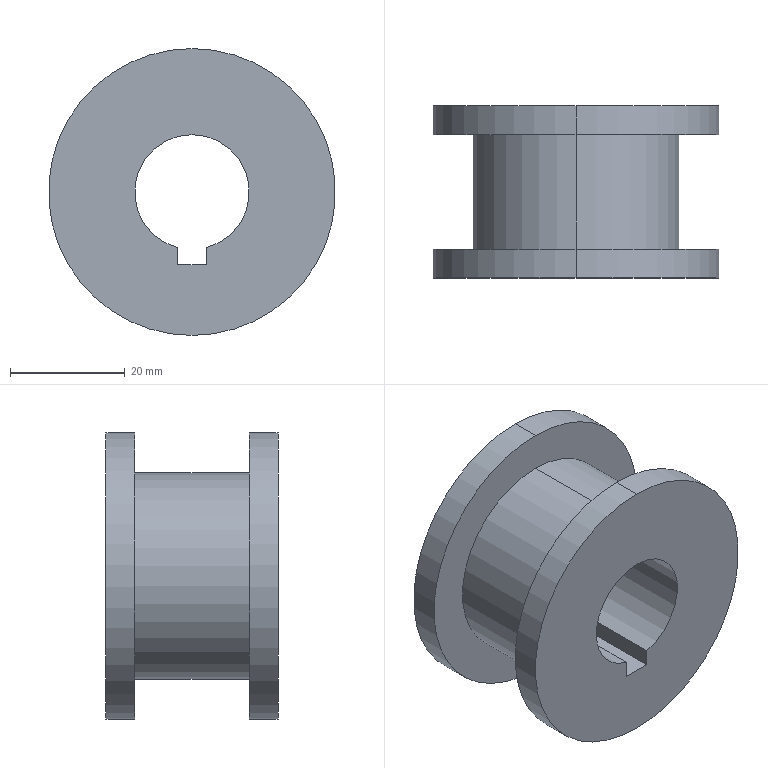Part | SolidWorks | features ICE 1, Revolution 1 | 1 solid | 15 faces | box 50 x 30 x 50 mm | volume 30150 mm3 | cylinder 8 | plane 7 | commonest cylinder face diameters 50 x4 20 x2 36 x2
STEP:
#1=CARTESIAN_POINT('',(0.,-5.,25.));
#2=VERTEX_POINT('',#1);
#3=CARTESIAN_POINT('',(0.,-5.,-25.));
#4=VERTEX_POINT('',#3);
#5=CARTESIAN_POINT('',(0.,-5.,0.));
#6=DIRECTION('',(0.,1.,0.));
#7=DIRECTION('',(0.,0.,1.));
#8=AXIS2_PLACEMENT_3D('',#5,#6,#7);
#9=CIRCLE('',#8,25.);
#10=EDGE_CURVE('',#2,#4,#9,.T.);
#11=ORIENTED_EDGE('',*,*,#10,.T.);
#12=CARTESIAN_POINT('',(0.,0.,-25.));
#13=VERTEX_POINT('',#12);
#14=CARTESIAN_POINT('',(0.,76.759,-25.));
#15=DIRECTION('',(0.,1.,0.));
#16=VECTOR('',#15,1000.);
#17=LINE('',#14,#16);
#18=EDGE_CURVE('',#4,#13,#17,.T.);
#19=ORIENTED_EDGE('',*,*,#18,.T.);
#20=CARTESIAN_POINT('',(0.,0.,25.));
#21=VERTEX_POINT('',#20);
#22=CARTESIAN_POINT('',(0.,0.,0.));
#23=DIRECTION('',(0.,1.,0.));
#24=DIRECTION('',(0.,0.,1.));
#25=AXIS2_PLACEMENT_3D('',#22,#23,#24);
#26=CIRCLE('',#25,25.);
#27=EDGE_CURVE('',#21,#13,#26,.T.);
#28=ORIENTED_EDGE('',*,*,#27,.F.);
#29=CARTESIAN_POINT('',(0.,76.759,25.));
#30=DIRECTION('',(0.,1.,0.));
#31=VECTOR('',#30,1000.);
#32=LINE('',#29,#31);
#33=EDGE_CURVE('',#2,#21,#32,.T.);
#34=ORIENTED_EDGE('',*,*,#33,.F.);
#35=EDGE_LOOP('',(#11,#19,#28,#34));
#36=FACE_OUTER_BOUND('',#35,.T.);
#37=CARTESIAN_POINT('',(0.,76.759,0.));
#38=DIRECTION('',(0.,1.,0.));
#39=DIRECTION('',(0.,0.,1.));
#40=AXIS2_PLACEMENT_3D('',#37,#38,#39);
#41=CYLINDRICAL_SURFACE('',#40,25.);
#42=ADVANCED_FACE('',(#36),#41,.T.);
#43=CARTESIAN_POINT('',(0.,-25.,18.));
#44=VERTEX_POINT('',#43);
#45=CARTESIAN_POINT('',(0.,-25.,-18.));
#46=VERTEX_POINT('',#45);
#47=CARTESIAN_POINT('',(0.,-25.,0.));
#48=DIRECTION('',(0.,1.,0.));
#49=DIRECTION('',(0.,0.,1.));
#50=AXIS2_PLACEMENT_3D('',#47,#48,#49);
#51=CIRCLE('',#50,18.);
#52=EDGE_CURVE('',#44,#46,#51,.T.);
#53=ORIENTED_EDGE('',*,*,#52,.T.);
#54=CARTESIAN_POINT('',(0.,-5.,-18.));
#55=VERTEX_POINT('',#54);
#56=CARTESIAN_POINT('',(0.,76.759,-18.));
#57=DIRECTION('',(0.,1.,0.));
#58=VECTOR('',#57,1000.);
#59=LINE('',#56,#58);
#60=EDGE_CURVE('',#46,#55,#59,.T.);
#61=ORIENTED_EDGE('',*,*,#60,.T.);
#62=CARTESIAN_POINT('',(0.,-5.,18.));
#63=VERTEX_POINT('',#62);
#64=CARTESIAN_POINT('',(0.,-5.,0.));
#65=DIRECTION('',(0.,1.,0.));
#66=DIRECTION('',(0.,0.,1.));
#67=AXIS2_PLACEMENT_3D('',#64,#65,#66);
#68=CIRCLE('',#67,18.);
#69=EDGE_CURVE('',#63,#55,#68,.T.);
#70=ORIENTED_EDGE('',*,*,#69,.F.);
#71=CARTESIAN_POINT('',(0.,76.759,18.));
#72=DIRECTION('',(0.,1.,0.));
#73=VECTOR('',#72,1000.);
#74=LINE('',#71,#73);
#75=EDGE_CURVE('',#44,#63,#74,.T.);
#76=ORIENTED_EDGE('',*,*,#75,.F.);
#77=EDGE_LOOP('',(#53,#61,#70,#76));
#78=FACE_OUTER_BOUND('',#77,.T.);
#79=CARTESIAN_POINT('',(0.,76.759,0.));
#80=DIRECTION('',(0.,1.,0.));
#81=DIRECTION('',(0.,0.,1.));
#82=AXIS2_PLACEMENT_3D('',#79,#80,#81);
#83=CYLINDRICAL_SURFACE('',#82,18.);
#84=ADVANCED_FACE('',(#78),#83,.T.);
#85=CARTESIAN_POINT('',(0.,-30.,25.));
#86=VERTEX_POINT('',#85);
#87=CARTESIAN_POINT('',(0.,-30.,-25.));
#88=VERTEX_POINT('',#87);
#89=CARTESIAN_POINT('',(0.,-30.,0.));
#90=DIRECTION('',(0.,1.,0.));
#91=DIRECTION('',(0.,0.,1.));
#92=AXIS2_PLACEMENT_3D('',#89,#90,#91);
#93=CIRCLE('',#92,25.);
#94=EDGE_CURVE('',#86,#88,#93,.T.);
#95=ORIENTED_EDGE('',*,*,#94,.T.);
#96=CARTESIAN_POINT('',(0.,-25.,-25.));
#97=VERTEX_POINT('',#96);
#98=CARTESIAN_POINT('',(0.,76.759,-25.));
#99=DIRECTION('',(0.,1.,0.));
#100=VECTOR('',#99,1000.);
#101=LINE('',#98,#100);
#102=EDGE_CURVE('',#88,#97,#101,.T.);
#103=ORIENTED_EDGE('',*,*,#102,.T.);
#104=CARTESIAN_POINT('',(0.,-25.,25.));
#105=VERTEX_POINT('',#104);
#106=CARTESIAN_POINT('',(0.,-25.,0.));
#107=DIRECTION('',(0.,1.,0.));
#108=DIRECTION('',(0.,0.,1.));
#109=AXIS2_PLACEMENT_3D('',#106,#107,#108);
#110=CIRCLE('',#109,25.);
#111=EDGE_CURVE('',#105,#97,#110,.T.);
#112=ORIENTED_EDGE('',*,*,#111,.F.);
#113=CARTESIAN_POINT('',(0.,76.759,25.));
#114=DIRECTION('',(0.,1.,0.));
#115=VECTOR('',#114,1000.);
#116=LINE('',#113,#115);
#117=EDGE_CURVE('',#86,#105,#116,.T.);
#118=ORIENTED_EDGE('',*,*,#117,.F.);
#119=EDGE_LOOP('',(#95,#103,#112,#118));
#120=FACE_OUTER_BOUND('',#119,.T.);
#121=CARTESIAN_POINT('',(0.,76.759,0.));
#122=DIRECTION('',(0.,1.,0.));
#123=DIRECTION('',(0.,0.,1.));
#124=AXIS2_PLACEMENT_3D('',#121,#122,#123);
#125=CYLINDRICAL_SURFACE('',#124,25.);
#126=ADVANCED_FACE('',(#120),#125,.T.);
#127=CARTESIAN_POINT('',(0.,-30.,10.));
#128=VERTEX_POINT('',#127);
#129=CARTESIAN_POINT('',(2.5,-30.,-9.682));
#130=VERTEX_POINT('',#129);
#131=CARTESIAN_POINT('',(0.,-30.,0.));
#132=DIRECTION('',(0.,1.,0.));
#133=DIRECTION('',(0.,0.,1.));
#134=AXIS2_PLACEMENT_3D('',#131,#132,#133);
#135=CIRCLE('',#134,10.);
#136=EDGE_CURVE('',#128,#130,#135,.T.);
#137=ORIENTED_EDGE('',*,*,#136,.F.);
#138=CARTESIAN_POINT('',(0.,0.,10.));
#139=VERTEX_POINT('',#138);
#140=CARTESIAN_POINT('',(0.,76.759,10.));
#141=DIRECTION('',(0.,1.,0.));
#142=VECTOR('',#141,1000.);
#143=LINE('',#140,#142);
#144=EDGE_CURVE('',#128,#139,#143,.T.);
#145=ORIENTED_EDGE('',*,*,#144,.T.);
#146=CARTESIAN_POINT('',(2.5,0.,-9.682));
#147=VERTEX_POINT('',#146);
#148=CARTESIAN_POINT('',(0.,0.,0.));
#149=DIRECTION('',(0.,1.,0.));
#150=DIRECTION('',(0.,0.,1.));
#151=AXIS2_PLACEMENT_3D('',#148,#149,#150);
#152=CIRCLE('',#151,10.);
#153=EDGE_CURVE('',#139,#147,#152,.T.);
#154=ORIENTED_EDGE('',*,*,#153,.T.);
#155=CARTESIAN_POINT('',(2.5,-30.,-9.682));
#156=DIRECTION('',(0.,1.,0.));
#157=VECTOR('',#156,1000.);
#158=LINE('',#155,#157);
#159=EDGE_CURVE('',#130,#147,#158,.T.);
#160=ORIENTED_EDGE('',*,*,#159,.F.);
#161=EDGE_LOOP('',(#137,#145,#154,#160));
#162=FACE_OUTER_BOUND('',#161,.T.);
#163=CARTESIAN_POINT('',(0.,76.759,0.));
#164=DIRECTION('',(0.,1.,0.));
#165=DIRECTION('',(0.,0.,1.));
#166=AXIS2_PLACEMENT_3D('',#163,#164,#165);
#167=CYLINDRICAL_SURFACE('',#166,10.);
#168=ADVANCED_FACE('',(#162),#167,.F.);
#169=CARTESIAN_POINT('',(2.5,0.,-12.682));
#170=VERTEX_POINT('',#169);
#171=CARTESIAN_POINT('',(2.5,0.,-12.682));
#172=DIRECTION('',(0.,0.,-1.));
#173=VECTOR('',#172,1000.);
#174=LINE('',#171,#173);
#175=EDGE_CURVE('',#147,#170,#174,.T.);
#176=ORIENTED_EDGE('',*,*,#175,.F.);
#177=ORIENTED_EDGE('',*,*,#153,.F.);
#178=CARTESIAN_POINT('',(-2.5,0.,-9.682));
#179=VERTEX_POINT('',#178);
#180=CARTESIAN_POINT('',(0.,0.,0.));
#181=DIRECTION('',(0.,1.,0.));
#182=DIRECTION('',(0.,0.,1.));
#183=AXIS2_PLACEMENT_3D('',#180,#181,#182);
#184=CIRCLE('',#183,10.);
#185=EDGE_CURVE('',#179,#139,#184,.T.);
#186=ORIENTED_EDGE('',*,*,#185,.F.);
#187=CARTESIAN_POINT('',(-2.5,0.,-12.682));
#188=VERTEX_POINT('',#187);
#189=CARTESIAN_POINT('',(-2.5,0.,-12.682));
#190=DIRECTION('',(0.,0.,1.));
#191=VECTOR('',#190,1000.);
#192=LINE('',#189,#191);
#193=EDGE_CURVE('',#188,#179,#192,.T.);
#194=ORIENTED_EDGE('',*,*,#193,.F.);
#195=CARTESIAN_POINT('',(-2.5,0.,-12.682));
#196=DIRECTION('',(-1.,0.,0.));
#197=VECTOR('',#196,1000.);
#198=LINE('',#195,#197);
#199=EDGE_CURVE('',#170,#188,#198,.T.);
#200=ORIENTED_EDGE('',*,*,#199,.F.);
#201=EDGE_LOOP('',(#176,#177,#186,#194,#200));
#202=FACE_BOUND('',#201,.T.);
#203=ORIENTED_EDGE('',*,*,#27,.T.);
#204=CARTESIAN_POINT('',(0.,0.,0.));
#205=DIRECTION('',(0.,1.,0.));
#206=DIRECTION('',(0.,0.,1.));
#207=AXIS2_PLACEMENT_3D('',#204,#205,#206);
#208=CIRCLE('',#207,25.);
#209=EDGE_CURVE('',#13,#21,#208,.T.);
#210=ORIENTED_EDGE('',*,*,#209,.T.);
#211=EDGE_LOOP('',(#203,#210));
#212=FACE_OUTER_BOUND('',#211,.T.);
#213=CARTESIAN_POINT('',(-25.,0.,0.));
#214=DIRECTION('',(0.,1.,0.));
#215=DIRECTION('',(0.,0.,1.));
#216=AXIS2_PLACEMENT_3D('',#213,#214,#215);
#217=PLANE('',#216);
#218=ADVANCED_FACE('',(#202,#212),#217,.T.);
#219=ORIENTED_EDGE('',*,*,#144,.F.);
#220=CARTESIAN_POINT('',(-2.5,-30.,-9.682));
#221=VERTEX_POINT('',#220);
#222=CARTESIAN_POINT('',(0.,-30.,0.));
#223=DIRECTION('',(0.,1.,0.));
#224=DIRECTION('',(0.,0.,1.));
#225=AXIS2_PLACEMENT_3D('',#222,#223,#224);
#226=CIRCLE('',#225,10.);
#227=EDGE_CURVE('',#221,#128,#226,.T.);
#228=ORIENTED_EDGE('',*,*,#227,.F.);
#229=CARTESIAN_POINT('',(-2.5,-30.,-9.682));
#230=DIRECTION('',(0.,1.,0.));
#231=VECTOR('',#230,1000.);
#232=LINE('',#229,#231);
#233=EDGE_CURVE('',#221,#179,#232,.T.);
#234=ORIENTED_EDGE('',*,*,#233,.T.);
#235=ORIENTED_EDGE('',*,*,#185,.T.);
#236=EDGE_LOOP('',(#219,#228,#234,#235));
#237=FACE_OUTER_BOUND('',#236,.T.);
#238=CARTESIAN_POINT('',(0.,76.759,0.));
#239=DIRECTION('',(0.,1.,0.));
#240=DIRECTION('',(0.,0.,1.));
#241=AXIS2_PLACEMENT_3D('',#238,#239,#240);
#242=CYLINDRICAL_SURFACE('',#241,10.);
#243=ADVANCED_FACE('',(#237),#242,.F.);
#244=CARTESIAN_POINT('',(2.5,-30.,-12.682));
#245=VERTEX_POINT('',#244);
#246=CARTESIAN_POINT('',(2.5,-30.,-12.682));
#247=DIRECTION('',(0.,0.,-1.));
#248=VECTOR('',#247,1000.);
#249=LINE('',#246,#248);
#250=EDGE_CURVE('',#130,#245,#249,.T.);
#251=ORIENTED_EDGE('',*,*,#250,.T.);
#252=CARTESIAN_POINT('',(-2.5,-30.,-12.682));
#253=VERTEX_POINT('',#252);
#254=CARTESIAN_POINT('',(-2.5,-30.,-12.682));
#255=DIRECTION('',(-1.,0.,0.));
#256=VECTOR('',#255,1000.);
#257=LINE('',#254,#256);
#258=EDGE_CURVE('',#245,#253,#257,.T.);
#259=ORIENTED_EDGE('',*,*,#258,.T.);
#260=CARTESIAN_POINT('',(-2.5,-30.,-12.682));
#261=DIRECTION('',(0.,0.,1.));
#262=VECTOR('',#261,1000.);
#263=LINE('',#260,#262);
#264=EDGE_CURVE('',#253,#221,#263,.T.);
#265=ORIENTED_EDGE('',*,*,#264,.T.);
#266=ORIENTED_EDGE('',*,*,#227,.T.);
#267=ORIENTED_EDGE('',*,*,#136,.T.);
#268=EDGE_LOOP('',(#251,#259,#265,#266,#267));
#269=FACE_BOUND('',#268,.T.);
#270=ORIENTED_EDGE('',*,*,#94,.F.);
#271=CARTESIAN_POINT('',(0.,-30.,0.));
#272=DIRECTION('',(0.,1.,0.));
#273=DIRECTION('',(0.,0.,1.));
#274=AXIS2_PLACEMENT_3D('',#271,#272,#273);
#275=CIRCLE('',#274,25.);
#276=EDGE_CURVE('',#88,#86,#275,.T.);
#277=ORIENTED_EDGE('',*,*,#276,.F.);
#278=EDGE_LOOP('',(#270,#277));
#279=FACE_OUTER_BOUND('',#278,.T.);
#280=CARTESIAN_POINT('',(-10.,-30.,0.));
#281=DIRECTION('',(0.,-1.,0.));
#282=DIRECTION('',(0.,0.,-1.));
#283=AXIS2_PLACEMENT_3D('',#280,#281,#282);
#284=PLANE('',#283);
#285=ADVANCED_FACE('',(#269,#279),#284,.T.);
#286=ORIENTED_EDGE('',*,*,#102,.F.);
#287=ORIENTED_EDGE('',*,*,#276,.T.);
#288=ORIENTED_EDGE('',*,*,#117,.T.);
#289=CARTESIAN_POINT('',(0.,-25.,0.));
#290=DIRECTION('',(0.,1.,0.));
#291=DIRECTION('',(0.,0.,1.));
#292=AXIS2_PLACEMENT_3D('',#289,#290,#291);
#293=CIRCLE('',#292,25.);
#294=EDGE_CURVE('',#97,#105,#293,.T.);
#295=ORIENTED_EDGE('',*,*,#294,.F.);
#296=EDGE_LOOP('',(#286,#287,#288,#295));
#297=FACE_OUTER_BOUND('',#296,.T.);
#298=CARTESIAN_POINT('',(0.,76.759,0.));
#299=DIRECTION('',(0.,1.,0.));
#300=DIRECTION('',(0.,0.,1.));
#301=AXIS2_PLACEMENT_3D('',#298,#299,#300);
#302=CYLINDRICAL_SURFACE('',#301,25.);
#303=ADVANCED_FACE('',(#297),#302,.T.);
#304=ORIENTED_EDGE('',*,*,#111,.T.);
#305=ORIENTED_EDGE('',*,*,#294,.T.);
#306=EDGE_LOOP('',(#304,#305));
#307=FACE_OUTER_BOUND('',#306,.T.);
#308=ORIENTED_EDGE('',*,*,#52,.F.);
#309=CARTESIAN_POINT('',(0.,-25.,0.));
#310=DIRECTION('',(0.,1.,0.));
#311=DIRECTION('',(0.,0.,1.));
#312=AXIS2_PLACEMENT_3D('',#309,#310,#311);
#313=CIRCLE('',#312,18.);
#314=EDGE_CURVE('',#46,#44,#313,.T.);
#315=ORIENTED_EDGE('',*,*,#314,.F.);
#316=EDGE_LOOP('',(#308,#315));
#317=FACE_BOUND('',#316,.T.);
#318=CARTESIAN_POINT('',(-25.,-25.,0.));
#319=DIRECTION('',(0.,1.,0.));
#320=DIRECTION('',(0.,0.,1.));
#321=AXIS2_PLACEMENT_3D('',#318,#319,#320);
#322=PLANE('',#321);
#323=ADVANCED_FACE('',(#307,#317),#322,.T.);
#324=ORIENTED_EDGE('',*,*,#60,.F.);
#325=ORIENTED_EDGE('',*,*,#314,.T.);
#326=ORIENTED_EDGE('',*,*,#75,.T.);
#327=CARTESIAN_POINT('',(0.,-5.,0.));
#328=DIRECTION('',(0.,1.,0.));
#329=DIRECTION('',(0.,0.,1.));
#330=AXIS2_PLACEMENT_3D('',#327,#328,#329);
#331=CIRCLE('',#330,18.);
#332=EDGE_CURVE('',#55,#63,#331,.T.);
#333=ORIENTED_EDGE('',*,*,#332,.F.);
#334=EDGE_LOOP('',(#324,#325,#326,#333));
#335=FACE_OUTER_BOUND('',#334,.T.);
#336=CARTESIAN_POINT('',(0.,76.759,0.));
#337=DIRECTION('',(0.,1.,0.));
#338=DIRECTION('',(0.,0.,1.));
#339=AXIS2_PLACEMENT_3D('',#336,#337,#338);
#340=CYLINDRICAL_SURFACE('',#339,18.);
#341=ADVANCED_FACE('',(#335),#340,.T.);
#342=ORIENTED_EDGE('',*,*,#69,.T.);
#343=ORIENTED_EDGE('',*,*,#332,.T.);
#344=EDGE_LOOP('',(#342,#343));
#345=FACE_BOUND('',#344,.T.);
#346=ORIENTED_EDGE('',*,*,#10,.F.);
#347=CARTESIAN_POINT('',(0.,-5.,0.));
#348=DIRECTION('',(0.,1.,0.));
#349=DIRECTION('',(0.,0.,1.));
#350=AXIS2_PLACEMENT_3D('',#347,#348,#349);
#351=CIRCLE('',#350,25.);
#352=EDGE_CURVE('',#4,#2,#351,.T.);
#353=ORIENTED_EDGE('',*,*,#352,.F.);
#354=EDGE_LOOP('',(#346,#353));
#355=FACE_OUTER_BOUND('',#354,.T.);
#356=CARTESIAN_POINT('',(-18.,-5.,0.));
#357=DIRECTION('',(0.,-1.,0.));
#358=DIRECTION('',(0.,0.,-1.));
#359=AXIS2_PLACEMENT_3D('',#356,#357,#358);
#360=PLANE('',#359);
#361=ADVANCED_FACE('',(#345,#355),#360,.T.);
#362=ORIENTED_EDGE('',*,*,#18,.F.);
#363=ORIENTED_EDGE('',*,*,#352,.T.);
#364=ORIENTED_EDGE('',*,*,#33,.T.);
#365=ORIENTED_EDGE('',*,*,#209,.F.);
#366=EDGE_LOOP('',(#362,#363,#364,#365));
#367=FACE_OUTER_BOUND('',#366,.T.);
#368=CARTESIAN_POINT('',(0.,76.759,0.));
#369=DIRECTION('',(0.,1.,0.));
#370=DIRECTION('',(0.,0.,1.));
#371=AXIS2_PLACEMENT_3D('',#368,#369,#370);
#372=CYLINDRICAL_SURFACE('',#371,25.);
#373=ADVANCED_FACE('',(#367),#372,.T.);
#374=ORIENTED_EDGE('',*,*,#199,.T.);
#375=CARTESIAN_POINT('',(-2.5,-30.,-12.682));
#376=DIRECTION('',(0.,1.,0.));
#377=VECTOR('',#376,1000.);
#378=LINE('',#375,#377);
#379=EDGE_CURVE('',#253,#188,#378,.T.);
#380=ORIENTED_EDGE('',*,*,#379,.F.);
#381=ORIENTED_EDGE('',*,*,#258,.F.);
#382=CARTESIAN_POINT('',(2.5,-30.,-12.682));
#383=DIRECTION('',(0.,1.,0.));
#384=VECTOR('',#383,1000.);
#385=LINE('',#382,#384);
#386=EDGE_CURVE('',#245,#170,#385,.T.);
#387=ORIENTED_EDGE('',*,*,#386,.T.);
#388=EDGE_LOOP('',(#374,#380,#381,#387));
#389=FACE_OUTER_BOUND('',#388,.T.);
#390=CARTESIAN_POINT('',(-2.5,-30.,-12.682));
#391=DIRECTION('',(0.,0.,-1.));
#392=DIRECTION('',(-1.,0.,0.));
#393=AXIS2_PLACEMENT_3D('',#390,#391,#392);
#394=PLANE('',#393);
#395=ADVANCED_FACE('',(#389),#394,.F.);
#396=ORIENTED_EDGE('',*,*,#175,.T.);
#397=ORIENTED_EDGE('',*,*,#386,.F.);
#398=ORIENTED_EDGE('',*,*,#250,.F.);
#399=ORIENTED_EDGE('',*,*,#159,.T.);
#400=EDGE_LOOP('',(#396,#397,#398,#399));
#401=FACE_OUTER_BOUND('',#400,.T.);
#402=CARTESIAN_POINT('',(2.5,-30.,-12.682));
#403=DIRECTION('',(1.,0.,0.));
#404=DIRECTION('',(0.,0.,-1.));
#405=AXIS2_PLACEMENT_3D('',#402,#403,#404);
#406=PLANE('',#405);
#407=ADVANCED_FACE('',(#401),#406,.F.);
#408=ORIENTED_EDGE('',*,*,#193,.T.);
#409=ORIENTED_EDGE('',*,*,#233,.F.);
#410=ORIENTED_EDGE('',*,*,#264,.F.);
#411=ORIENTED_EDGE('',*,*,#379,.T.);
#412=EDGE_LOOP('',(#408,#409,#410,#411));
#413=FACE_OUTER_BOUND('',#412,.T.);
#414=CARTESIAN_POINT('',(-2.5,-30.,-12.682));
#415=DIRECTION('',(-1.,0.,0.));
#416=DIRECTION('',(0.,0.,1.));
#417=AXIS2_PLACEMENT_3D('',#414,#415,#416);
#418=PLANE('',#417);
#419=ADVANCED_FACE('',(#413),#418,.F.);
#420=CLOSED_SHELL('',(#42,#84,#126,#168,#218,#243,#285,#303,#323,#341,#361,#373,#395,#407,#419));
#421=MANIFOLD_SOLID_BREP('',#420);
#422=CARTESIAN_POINT('',(0.,0.,0.));
#423=DIRECTION('',(0.,0.,1.));
#424=DIRECTION('',(1.,0.,0.));
#425=AXIS2_PLACEMENT_3D('',#422,#423,#424);
#426=(LENGTH_UNIT()NAMED_UNIT(*)SI_UNIT(.MILLI.,.METRE.));
#427=UNCERTAINTY_MEASURE_WITH_UNIT(LENGTH_MEASURE(0.00001),#426,'','');
#428=(NAMED_UNIT(*)PLANE_ANGLE_UNIT()SI_UNIT($,.RADIAN.));
#429=(NAMED_UNIT(*)SI_UNIT($,.STERADIAN.)SOLID_ANGLE_UNIT());
#430=(GEOMETRIC_REPRESENTATION_CONTEXT(3)GLOBAL_UNCERTAINTY_ASSIGNED_CONTEXT((#427))GLOBAL_UNIT_ASSIGNED_CONTEXT((#426,#428,#429))REPRESENTATION_CONTEXT('',''));
#431=ADVANCED_BREP_SHAPE_REPRESENTATION('',(#421,#425),#430);